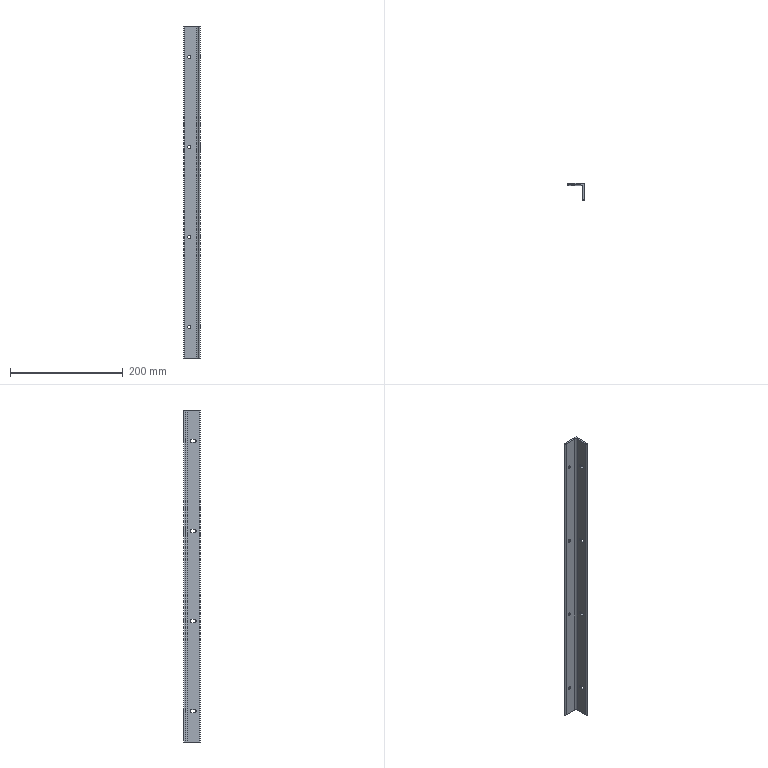Part | STEP file | 0228_207_Bracket | 1 solid | 35 faces | box 30 x 30 x 590 mm | volume 100045 mm3 | cylinder 19 | plane 16 | commonest cylinder face diameters 5.5 x16 4.5 x2 6.5 x1